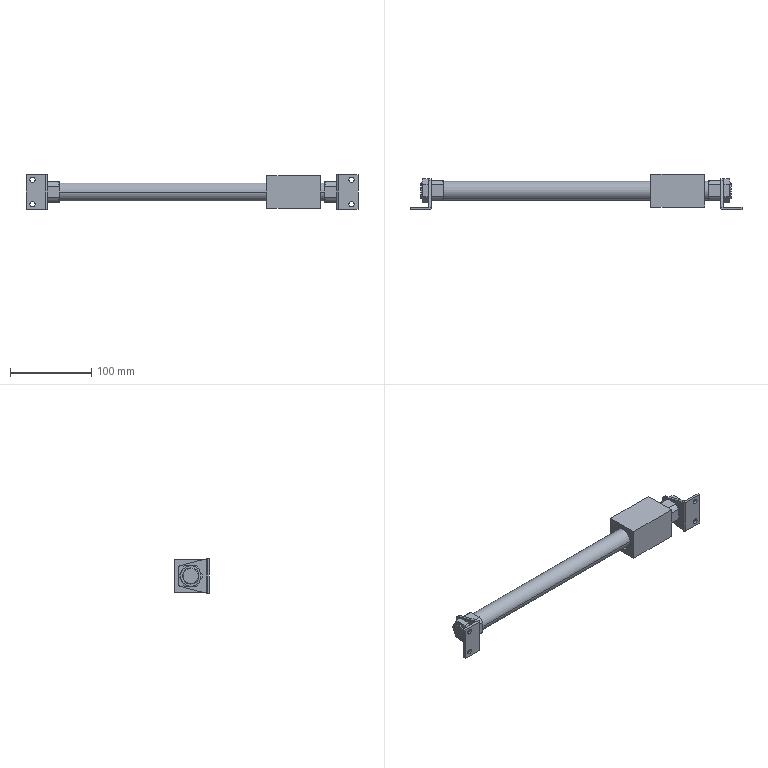Part | SolidWorks | 6 solids | 211 faces | box 408 x 43 x 43 mm | volume 151257 mm3 | cylinder 80 | plane 69 | cone 46 | spline 16 | commonest cylinder face diameters 2.5 x8 4 x8 6.5 x8 20 x8 29 x8 3 x6